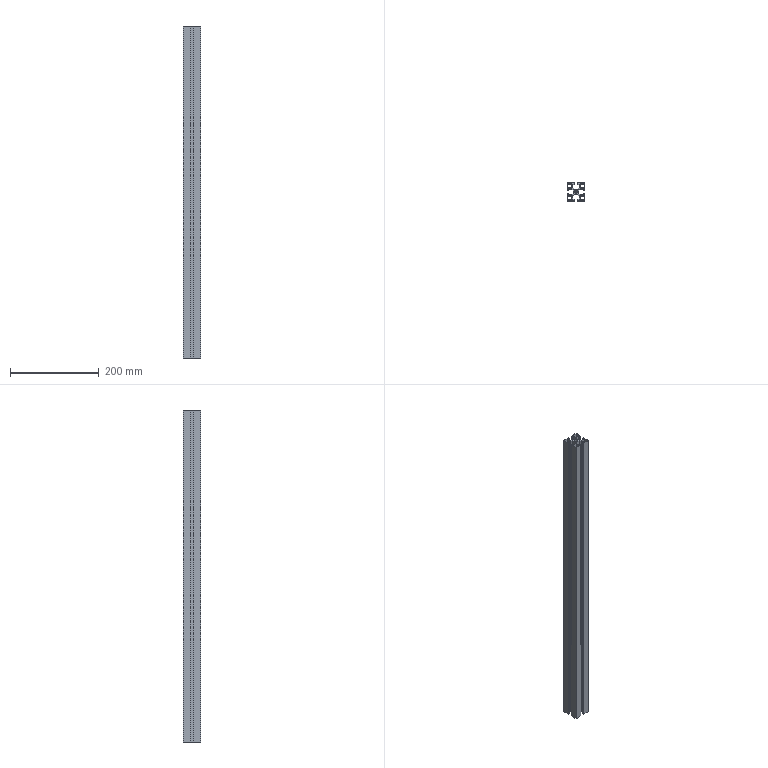Part | STEP file | 40_40_470_1-2 | 1 solid | 64 faces | box 40 x 40 x 750 mm | volume 393557 mm3 | plane 62 | cylinder 2 | commonest cylinder face diameters 6.8 x2